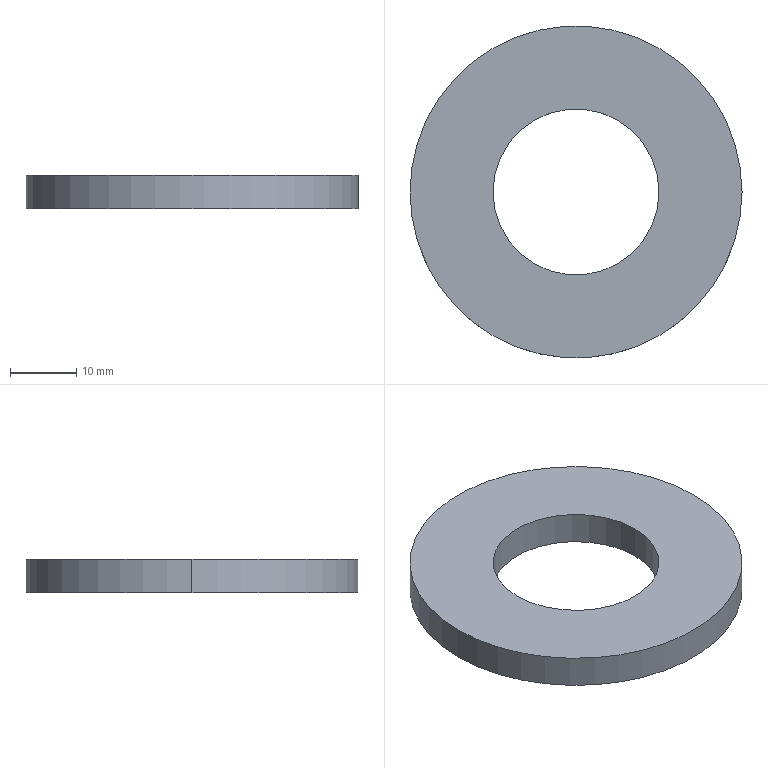Part | SolidWorks | features Cut 1, Extrusion 1 | 1 solid | 6 faces | box 50 x 50 x 5 mm | volume 7363 mm3 | cylinder 4 | plane 2 | commonest cylinder face diameters 25 x2 50 x2
STEP:
#1=CARTESIAN_POINT('',(-57.5,25.,2.5));
#2=VERTEX_POINT('',#1);
#3=CARTESIAN_POINT('',(-82.5,25.,2.5));
#4=VERTEX_POINT('',#3);
#5=CARTESIAN_POINT('',(-70.,25.,2.5));
#6=DIRECTION('',(0.,0.,-1.));
#7=DIRECTION('',(-1.,0.,0.));
#8=AXIS2_PLACEMENT_3D('',#5,#6,#7);
#9=CIRCLE('',#8,12.5);
#10=EDGE_CURVE('',#2,#4,#9,.T.);
#11=ORIENTED_EDGE('',*,*,#10,.F.);
#12=CARTESIAN_POINT('',(-57.5,25.,-2.5));
#13=VERTEX_POINT('',#12);
#14=CARTESIAN_POINT('',(-57.5,25.,2.5));
#15=DIRECTION('',(0.,0.,-1.));
#16=VECTOR('',#15,1000.);
#17=LINE('',#14,#16);
#18=EDGE_CURVE('',#2,#13,#17,.T.);
#19=ORIENTED_EDGE('',*,*,#18,.T.);
#20=CARTESIAN_POINT('',(-82.5,25.,-2.5));
#21=VERTEX_POINT('',#20);
#22=CARTESIAN_POINT('',(-70.,25.,-2.5));
#23=DIRECTION('',(0.,0.,-1.));
#24=DIRECTION('',(-1.,0.,0.));
#25=AXIS2_PLACEMENT_3D('',#22,#23,#24);
#26=CIRCLE('',#25,12.5);
#27=EDGE_CURVE('',#13,#21,#26,.T.);
#28=ORIENTED_EDGE('',*,*,#27,.T.);
#29=CARTESIAN_POINT('',(-82.5,25.,2.5));
#30=DIRECTION('',(0.,0.,-1.));
#31=VECTOR('',#30,1000.);
#32=LINE('',#29,#31);
#33=EDGE_CURVE('',#4,#21,#32,.T.);
#34=ORIENTED_EDGE('',*,*,#33,.F.);
#35=EDGE_LOOP('',(#11,#19,#28,#34));
#36=FACE_OUTER_BOUND('',#35,.T.);
#37=CARTESIAN_POINT('',(-70.,25.,2.5));
#38=DIRECTION('',(0.,0.,-1.));
#39=DIRECTION('',(-1.,0.,0.));
#40=AXIS2_PLACEMENT_3D('',#37,#38,#39);
#41=CYLINDRICAL_SURFACE('',#40,12.5);
#42=ADVANCED_FACE('',(#36),#41,.F.);
#43=CARTESIAN_POINT('',(-45.,25.,2.5));
#44=VERTEX_POINT('',#43);
#45=CARTESIAN_POINT('',(-95.,25.,2.5));
#46=VERTEX_POINT('',#45);
#47=CARTESIAN_POINT('',(-70.,25.,2.5));
#48=DIRECTION('',(0.,0.,1.));
#49=DIRECTION('',(1.,0.,0.));
#50=AXIS2_PLACEMENT_3D('',#47,#48,#49);
#51=CIRCLE('',#50,25.);
#52=EDGE_CURVE('',#44,#46,#51,.T.);
#53=ORIENTED_EDGE('',*,*,#52,.F.);
#54=CARTESIAN_POINT('',(-45.,25.,-2.5));
#55=VERTEX_POINT('',#54);
#56=CARTESIAN_POINT('',(-45.,25.,2.5));
#57=DIRECTION('',(0.,0.,-1.));
#58=VECTOR('',#57,1000.);
#59=LINE('',#56,#58);
#60=EDGE_CURVE('',#44,#55,#59,.T.);
#61=ORIENTED_EDGE('',*,*,#60,.T.);
#62=CARTESIAN_POINT('',(-95.,25.,-2.5));
#63=VERTEX_POINT('',#62);
#64=CARTESIAN_POINT('',(-70.,25.,-2.5));
#65=DIRECTION('',(0.,0.,1.));
#66=DIRECTION('',(1.,0.,0.));
#67=AXIS2_PLACEMENT_3D('',#64,#65,#66);
#68=CIRCLE('',#67,25.);
#69=EDGE_CURVE('',#55,#63,#68,.T.);
#70=ORIENTED_EDGE('',*,*,#69,.T.);
#71=CARTESIAN_POINT('',(-95.,25.,2.5));
#72=DIRECTION('',(0.,0.,-1.));
#73=VECTOR('',#72,1000.);
#74=LINE('',#71,#73);
#75=EDGE_CURVE('',#46,#63,#74,.T.);
#76=ORIENTED_EDGE('',*,*,#75,.F.);
#77=EDGE_LOOP('',(#53,#61,#70,#76));
#78=FACE_OUTER_BOUND('',#77,.T.);
#79=CARTESIAN_POINT('',(-70.,25.,2.5));
#80=DIRECTION('',(0.,0.,-1.));
#81=DIRECTION('',(-1.,0.,0.));
#82=AXIS2_PLACEMENT_3D('',#79,#80,#81);
#83=CYLINDRICAL_SURFACE('',#82,25.);
#84=ADVANCED_FACE('',(#78),#83,.T.);
#85=ORIENTED_EDGE('',*,*,#60,.F.);
#86=CARTESIAN_POINT('',(-70.,25.,2.5));
#87=DIRECTION('',(0.,0.,1.));
#88=DIRECTION('',(1.,0.,0.));
#89=AXIS2_PLACEMENT_3D('',#86,#87,#88);
#90=CIRCLE('',#89,25.);
#91=EDGE_CURVE('',#46,#44,#90,.T.);
#92=ORIENTED_EDGE('',*,*,#91,.F.);
#93=ORIENTED_EDGE('',*,*,#75,.T.);
#94=CARTESIAN_POINT('',(-70.,25.,-2.5));
#95=DIRECTION('',(0.,0.,1.));
#96=DIRECTION('',(1.,0.,0.));
#97=AXIS2_PLACEMENT_3D('',#94,#95,#96);
#98=CIRCLE('',#97,25.);
#99=EDGE_CURVE('',#63,#55,#98,.T.);
#100=ORIENTED_EDGE('',*,*,#99,.T.);
#101=EDGE_LOOP('',(#85,#92,#93,#100));
#102=FACE_OUTER_BOUND('',#101,.T.);
#103=CARTESIAN_POINT('',(-70.,25.,2.5));
#104=DIRECTION('',(0.,0.,-1.));
#105=DIRECTION('',(-1.,0.,0.));
#106=AXIS2_PLACEMENT_3D('',#103,#104,#105);
#107=CYLINDRICAL_SURFACE('',#106,25.);
#108=ADVANCED_FACE('',(#102),#107,.T.);
#109=CARTESIAN_POINT('',(-70.,25.,2.5));
#110=DIRECTION('',(0.,0.,-1.));
#111=DIRECTION('',(-1.,0.,0.));
#112=AXIS2_PLACEMENT_3D('',#109,#110,#111);
#113=CIRCLE('',#112,12.5);
#114=EDGE_CURVE('',#4,#2,#113,.T.);
#115=ORIENTED_EDGE('',*,*,#114,.T.);
#116=ORIENTED_EDGE('',*,*,#10,.T.);
#117=EDGE_LOOP('',(#115,#116));
#118=FACE_BOUND('',#117,.T.);
#119=ORIENTED_EDGE('',*,*,#91,.T.);
#120=ORIENTED_EDGE('',*,*,#52,.T.);
#121=EDGE_LOOP('',(#119,#120));
#122=FACE_OUTER_BOUND('',#121,.T.);
#123=CARTESIAN_POINT('',(-70.,25.,2.5));
#124=DIRECTION('',(0.,0.,1.));
#125=DIRECTION('',(1.,0.,0.));
#126=AXIS2_PLACEMENT_3D('',#123,#124,#125);
#127=PLANE('',#126);
#128=ADVANCED_FACE('',(#118,#122),#127,.T.);
#129=CARTESIAN_POINT('',(-70.,25.,-2.5));
#130=DIRECTION('',(0.,0.,-1.));
#131=DIRECTION('',(-1.,0.,0.));
#132=AXIS2_PLACEMENT_3D('',#129,#130,#131);
#133=CIRCLE('',#132,12.5);
#134=EDGE_CURVE('',#21,#13,#133,.T.);
#135=ORIENTED_EDGE('',*,*,#134,.F.);
#136=ORIENTED_EDGE('',*,*,#27,.F.);
#137=EDGE_LOOP('',(#135,#136));
#138=FACE_BOUND('',#137,.T.);
#139=ORIENTED_EDGE('',*,*,#99,.F.);
#140=ORIENTED_EDGE('',*,*,#69,.F.);
#141=EDGE_LOOP('',(#139,#140));
#142=FACE_OUTER_BOUND('',#141,.T.);
#143=CARTESIAN_POINT('',(-70.,25.,-2.5));
#144=DIRECTION('',(0.,0.,1.));
#145=DIRECTION('',(1.,0.,0.));
#146=AXIS2_PLACEMENT_3D('',#143,#144,#145);
#147=PLANE('',#146);
#148=ADVANCED_FACE('',(#138,#142),#147,.F.);
#149=ORIENTED_EDGE('',*,*,#18,.F.);
#150=ORIENTED_EDGE('',*,*,#114,.F.);
#151=ORIENTED_EDGE('',*,*,#33,.T.);
#152=ORIENTED_EDGE('',*,*,#134,.T.);
#153=EDGE_LOOP('',(#149,#150,#151,#152));
#154=FACE_OUTER_BOUND('',#153,.T.);
#155=CARTESIAN_POINT('',(-70.,25.,2.5));
#156=DIRECTION('',(0.,0.,-1.));
#157=DIRECTION('',(-1.,0.,0.));
#158=AXIS2_PLACEMENT_3D('',#155,#156,#157);
#159=CYLINDRICAL_SURFACE('',#158,12.5);
#160=ADVANCED_FACE('',(#154),#159,.F.);
#161=CLOSED_SHELL('',(#42,#84,#108,#128,#148,#160));
#162=MANIFOLD_SOLID_BREP('',#161);
#163=CARTESIAN_POINT('',(0.,0.,0.));
#164=DIRECTION('',(0.,0.,1.));
#165=DIRECTION('',(1.,0.,0.));
#166=AXIS2_PLACEMENT_3D('',#163,#164,#165);
#167=(LENGTH_UNIT()NAMED_UNIT(*)SI_UNIT(.MILLI.,.METRE.));
#168=UNCERTAINTY_MEASURE_WITH_UNIT(LENGTH_MEASURE(0.00001),#167,'','');
#169=(NAMED_UNIT(*)PLANE_ANGLE_UNIT()SI_UNIT($,.RADIAN.));
#170=(NAMED_UNIT(*)SI_UNIT($,.STERADIAN.)SOLID_ANGLE_UNIT());
#171=(GEOMETRIC_REPRESENTATION_CONTEXT(3)GLOBAL_UNCERTAINTY_ASSIGNED_CONTEXT((#168))GLOBAL_UNIT_ASSIGNED_CONTEXT((#167,#169,#170))REPRESENTATION_CONTEXT('',''));
#172=ADVANCED_BREP_SHAPE_REPRESENTATION('',(#162,#166),#171);